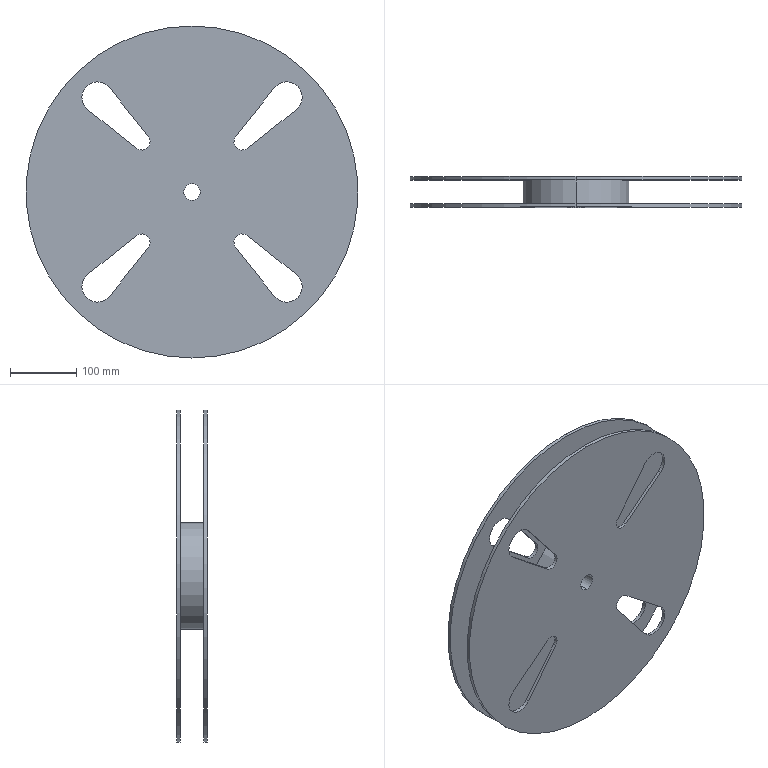Part | NX | 1 solid | 52 faces | box 500 x 46 x 500 mm | volume 2483215 mm3 | cylinder 32 | plane 20 | commonest cylinder face diameters 25 x14 47.051 x12 500 x4 160 x2